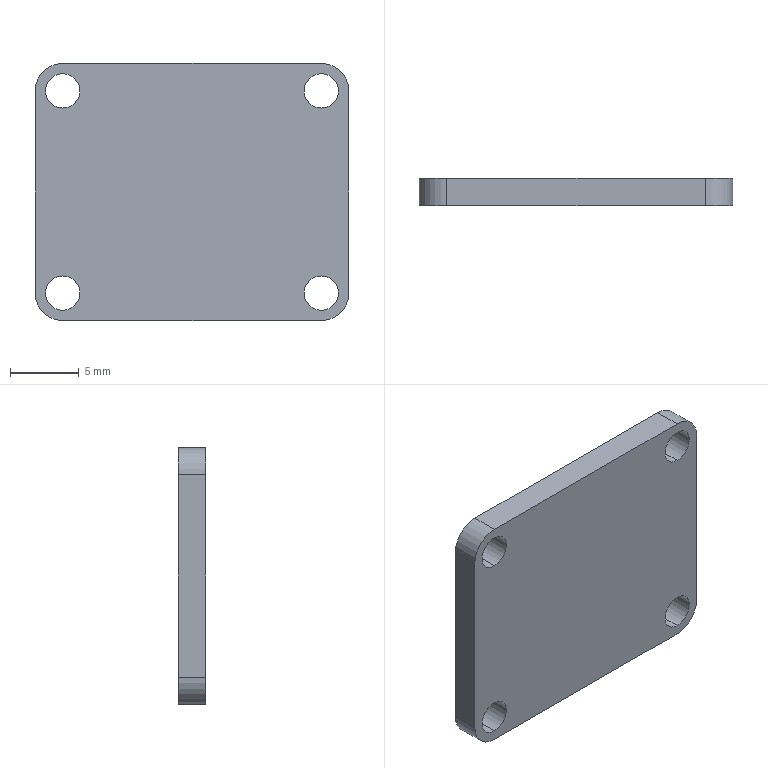Part | SolidWorks | features ICE 5, ExtruThin 1, Fillet 1 | 1 solid | 18 faces | box 22.8 x 2 x 18.7 mm | volume 806.583 mm3 | cylinder 12 | plane 6 | commonest cylinder face diameters 2.5 x8 4 x4
STEP:
#1=CARTESIAN_POINT('',(36.275,113.634,-14.95));
#2=VERTEX_POINT('',#1);
#3=CARTESIAN_POINT('',(36.275,113.634,-12.45));
#4=VERTEX_POINT('',#3);
#5=CARTESIAN_POINT('',(36.275,113.634,-13.7));
#6=DIRECTION('',(0.,1.,0.));
#7=DIRECTION('',(0.,0.,1.));
#8=AXIS2_PLACEMENT_3D('',#5,#6,#7);
#9=CIRCLE('',#8,1.25);
#10=EDGE_CURVE('',#2,#4,#9,.T.);
#11=ORIENTED_EDGE('',*,*,#10,.F.);
#12=CARTESIAN_POINT('',(36.275,115.634,-14.95));
#13=VERTEX_POINT('',#12);
#14=CARTESIAN_POINT('',(36.275,113.634,-14.95));
#15=DIRECTION('',(0.,1.,0.));
#16=VECTOR('',#15,1000.);
#17=LINE('',#14,#16);
#18=EDGE_CURVE('',#2,#13,#17,.T.);
#19=ORIENTED_EDGE('',*,*,#18,.T.);
#20=CARTESIAN_POINT('',(36.275,115.634,-12.45));
#21=VERTEX_POINT('',#20);
#22=CARTESIAN_POINT('',(36.275,115.634,-13.7));
#23=DIRECTION('',(0.,1.,0.));
#24=DIRECTION('',(0.,0.,1.));
#25=AXIS2_PLACEMENT_3D('',#22,#23,#24);
#26=CIRCLE('',#25,1.25);
#27=EDGE_CURVE('',#13,#21,#26,.T.);
#28=ORIENTED_EDGE('',*,*,#27,.T.);
#29=CARTESIAN_POINT('',(36.275,113.634,-12.45));
#30=DIRECTION('',(0.,1.,0.));
#31=VECTOR('',#30,1000.);
#32=LINE('',#29,#31);
#33=EDGE_CURVE('',#4,#21,#32,.T.);
#34=ORIENTED_EDGE('',*,*,#33,.F.);
#35=EDGE_LOOP('',(#11,#19,#28,#34));
#36=FACE_OUTER_BOUND('',#35,.T.);
#37=CARTESIAN_POINT('',(36.275,113.634,-13.7));
#38=DIRECTION('',(0.,1.,0.));
#39=DIRECTION('',(0.,0.,1.));
#40=AXIS2_PLACEMENT_3D('',#37,#38,#39);
#41=CYLINDRICAL_SURFACE('',#40,1.25);
#42=ADVANCED_FACE('',(#36),#41,.F.);
#43=CARTESIAN_POINT('',(36.275,113.634,-0.25));
#44=VERTEX_POINT('',#43);
#45=CARTESIAN_POINT('',(36.275,113.634,2.25));
#46=VERTEX_POINT('',#45);
#47=CARTESIAN_POINT('',(36.275,113.634,1.));
#48=DIRECTION('',(0.,1.,0.));
#49=DIRECTION('',(0.,0.,1.));
#50=AXIS2_PLACEMENT_3D('',#47,#48,#49);
#51=CIRCLE('',#50,1.25);
#52=EDGE_CURVE('',#44,#46,#51,.T.);
#53=ORIENTED_EDGE('',*,*,#52,.F.);
#54=CARTESIAN_POINT('',(36.275,115.634,-0.25));
#55=VERTEX_POINT('',#54);
#56=CARTESIAN_POINT('',(36.275,113.634,-0.25));
#57=DIRECTION('',(0.,1.,0.));
#58=VECTOR('',#57,1000.);
#59=LINE('',#56,#58);
#60=EDGE_CURVE('',#44,#55,#59,.T.);
#61=ORIENTED_EDGE('',*,*,#60,.T.);
#62=CARTESIAN_POINT('',(36.275,115.634,2.25));
#63=VERTEX_POINT('',#62);
#64=CARTESIAN_POINT('',(36.275,115.634,1.));
#65=DIRECTION('',(0.,1.,0.));
#66=DIRECTION('',(0.,0.,1.));
#67=AXIS2_PLACEMENT_3D('',#64,#65,#66);
#68=CIRCLE('',#67,1.25);
#69=EDGE_CURVE('',#55,#63,#68,.T.);
#70=ORIENTED_EDGE('',*,*,#69,.T.);
#71=CARTESIAN_POINT('',(36.275,113.634,2.25));
#72=DIRECTION('',(0.,1.,0.));
#73=VECTOR('',#72,1000.);
#74=LINE('',#71,#73);
#75=EDGE_CURVE('',#46,#63,#74,.T.);
#76=ORIENTED_EDGE('',*,*,#75,.F.);
#77=EDGE_LOOP('',(#53,#61,#70,#76));
#78=FACE_OUTER_BOUND('',#77,.T.);
#79=CARTESIAN_POINT('',(36.275,113.634,1.));
#80=DIRECTION('',(0.,1.,0.));
#81=DIRECTION('',(0.,0.,1.));
#82=AXIS2_PLACEMENT_3D('',#79,#80,#81);
#83=CYLINDRICAL_SURFACE('',#82,1.25);
#84=ADVANCED_FACE('',(#78),#83,.F.);
#85=CARTESIAN_POINT('',(55.075,113.634,-0.25));
#86=VERTEX_POINT('',#85);
#87=CARTESIAN_POINT('',(55.075,113.634,2.25));
#88=VERTEX_POINT('',#87);
#89=CARTESIAN_POINT('',(55.075,113.634,1.));
#90=DIRECTION('',(0.,1.,0.));
#91=DIRECTION('',(0.,0.,1.));
#92=AXIS2_PLACEMENT_3D('',#89,#90,#91);
#93=CIRCLE('',#92,1.25);
#94=EDGE_CURVE('',#86,#88,#93,.T.);
#95=ORIENTED_EDGE('',*,*,#94,.F.);
#96=CARTESIAN_POINT('',(55.075,115.634,-0.25));
#97=VERTEX_POINT('',#96);
#98=CARTESIAN_POINT('',(55.075,113.634,-0.25));
#99=DIRECTION('',(0.,1.,0.));
#100=VECTOR('',#99,1000.);
#101=LINE('',#98,#100);
#102=EDGE_CURVE('',#86,#97,#101,.T.);
#103=ORIENTED_EDGE('',*,*,#102,.T.);
#104=CARTESIAN_POINT('',(55.075,115.634,2.25));
#105=VERTEX_POINT('',#104);
#106=CARTESIAN_POINT('',(55.075,115.634,1.));
#107=DIRECTION('',(0.,1.,0.));
#108=DIRECTION('',(0.,0.,1.));
#109=AXIS2_PLACEMENT_3D('',#106,#107,#108);
#110=CIRCLE('',#109,1.25);
#111=EDGE_CURVE('',#97,#105,#110,.T.);
#112=ORIENTED_EDGE('',*,*,#111,.T.);
#113=CARTESIAN_POINT('',(55.075,113.634,2.25));
#114=DIRECTION('',(0.,1.,0.));
#115=VECTOR('',#114,1000.);
#116=LINE('',#113,#115);
#117=EDGE_CURVE('',#88,#105,#116,.T.);
#118=ORIENTED_EDGE('',*,*,#117,.F.);
#119=EDGE_LOOP('',(#95,#103,#112,#118));
#120=FACE_OUTER_BOUND('',#119,.T.);
#121=CARTESIAN_POINT('',(55.075,113.634,1.));
#122=DIRECTION('',(0.,1.,0.));
#123=DIRECTION('',(0.,0.,1.));
#124=AXIS2_PLACEMENT_3D('',#121,#122,#123);
#125=CYLINDRICAL_SURFACE('',#124,1.25);
#126=ADVANCED_FACE('',(#120),#125,.F.);
#127=CARTESIAN_POINT('',(55.075,113.634,-14.95));
#128=VERTEX_POINT('',#127);
#129=CARTESIAN_POINT('',(55.075,113.634,-12.45));
#130=VERTEX_POINT('',#129);
#131=CARTESIAN_POINT('',(55.075,113.634,-13.7));
#132=DIRECTION('',(0.,1.,0.));
#133=DIRECTION('',(0.,0.,1.));
#134=AXIS2_PLACEMENT_3D('',#131,#132,#133);
#135=CIRCLE('',#134,1.25);
#136=EDGE_CURVE('',#128,#130,#135,.T.);
#137=ORIENTED_EDGE('',*,*,#136,.F.);
#138=CARTESIAN_POINT('',(55.075,115.634,-14.95));
#139=VERTEX_POINT('',#138);
#140=CARTESIAN_POINT('',(55.075,113.634,-14.95));
#141=DIRECTION('',(0.,1.,0.));
#142=VECTOR('',#141,1000.);
#143=LINE('',#140,#142);
#144=EDGE_CURVE('',#128,#139,#143,.T.);
#145=ORIENTED_EDGE('',*,*,#144,.T.);
#146=CARTESIAN_POINT('',(55.075,115.634,-12.45));
#147=VERTEX_POINT('',#146);
#148=CARTESIAN_POINT('',(55.075,115.634,-13.7));
#149=DIRECTION('',(0.,1.,0.));
#150=DIRECTION('',(0.,0.,1.));
#151=AXIS2_PLACEMENT_3D('',#148,#149,#150);
#152=CIRCLE('',#151,1.25);
#153=EDGE_CURVE('',#139,#147,#152,.T.);
#154=ORIENTED_EDGE('',*,*,#153,.T.);
#155=CARTESIAN_POINT('',(55.075,113.634,-12.45));
#156=DIRECTION('',(0.,1.,0.));
#157=VECTOR('',#156,1000.);
#158=LINE('',#155,#157);
#159=EDGE_CURVE('',#130,#147,#158,.T.);
#160=ORIENTED_EDGE('',*,*,#159,.F.);
#161=EDGE_LOOP('',(#137,#145,#154,#160));
#162=FACE_OUTER_BOUND('',#161,.T.);
#163=CARTESIAN_POINT('',(55.075,113.634,-13.7));
#164=DIRECTION('',(0.,1.,0.));
#165=DIRECTION('',(0.,0.,1.));
#166=AXIS2_PLACEMENT_3D('',#163,#164,#165);
#167=CYLINDRICAL_SURFACE('',#166,1.25);
#168=ADVANCED_FACE('',(#162),#167,.F.);
#169=CARTESIAN_POINT('',(57.075,115.634,1.));
#170=VERTEX_POINT('',#169);
#171=CARTESIAN_POINT('',(57.075,115.634,-13.7));
#172=VERTEX_POINT('',#171);
#173=CARTESIAN_POINT('',(57.075,115.634,-15.7));
#174=DIRECTION('',(0.,0.,-1.));
#175=VECTOR('',#174,1000.);
#176=LINE('',#173,#175);
#177=EDGE_CURVE('',#170,#172,#176,.T.);
#178=ORIENTED_EDGE('',*,*,#177,.F.);
#179=CARTESIAN_POINT('',(57.075,113.634,1.));
#180=VERTEX_POINT('',#179);
#181=CARTESIAN_POINT('',(57.075,115.634,1.));
#182=DIRECTION('',(0.,-1.,0.));
#183=VECTOR('',#182,1000.);
#184=LINE('',#181,#183);
#185=EDGE_CURVE('',#170,#180,#184,.T.);
#186=ORIENTED_EDGE('',*,*,#185,.T.);
#187=CARTESIAN_POINT('',(57.075,113.634,-13.7));
#188=VERTEX_POINT('',#187);
#189=CARTESIAN_POINT('',(57.075,113.634,-15.7));
#190=DIRECTION('',(0.,0.,-1.));
#191=VECTOR('',#190,1000.);
#192=LINE('',#189,#191);
#193=EDGE_CURVE('',#180,#188,#192,.T.);
#194=ORIENTED_EDGE('',*,*,#193,.T.);
#195=CARTESIAN_POINT('',(57.075,115.634,-13.7));
#196=DIRECTION('',(0.,1.,0.));
#197=VECTOR('',#196,1000.);
#198=LINE('',#195,#197);
#199=EDGE_CURVE('',#188,#172,#198,.T.);
#200=ORIENTED_EDGE('',*,*,#199,.T.);
#201=EDGE_LOOP('',(#178,#186,#194,#200));
#202=FACE_OUTER_BOUND('',#201,.T.);
#203=CARTESIAN_POINT('',(57.075,115.634,-15.7));
#204=DIRECTION('',(-1.,0.,0.));
#205=DIRECTION('',(0.,0.,1.));
#206=AXIS2_PLACEMENT_3D('',#203,#204,#205);
#207=PLANE('',#206);
#208=ADVANCED_FACE('',(#202),#207,.F.);
#209=CARTESIAN_POINT('',(55.075,113.634,-15.7));
#210=VERTEX_POINT('',#209);
#211=CARTESIAN_POINT('',(36.275,113.634,-15.7));
#212=VERTEX_POINT('',#211);
#213=CARTESIAN_POINT('',(57.075,113.634,-15.7));
#214=DIRECTION('',(-1.,0.,0.));
#215=VECTOR('',#214,1000.);
#216=LINE('',#213,#215);
#217=EDGE_CURVE('',#210,#212,#216,.T.);
#218=ORIENTED_EDGE('',*,*,#217,.T.);
#219=CARTESIAN_POINT('',(36.275,115.634,-15.7));
#220=VERTEX_POINT('',#219);
#221=CARTESIAN_POINT('',(36.275,115.634,-15.7));
#222=DIRECTION('',(0.,1.,0.));
#223=VECTOR('',#222,1000.);
#224=LINE('',#221,#223);
#225=EDGE_CURVE('',#212,#220,#224,.T.);
#226=ORIENTED_EDGE('',*,*,#225,.T.);
#227=CARTESIAN_POINT('',(55.075,115.634,-15.7));
#228=VERTEX_POINT('',#227);
#229=CARTESIAN_POINT('',(57.075,115.634,-15.7));
#230=DIRECTION('',(-1.,0.,0.));
#231=VECTOR('',#230,1000.);
#232=LINE('',#229,#231);
#233=EDGE_CURVE('',#228,#220,#232,.T.);
#234=ORIENTED_EDGE('',*,*,#233,.F.);
#235=CARTESIAN_POINT('',(55.075,115.634,-15.7));
#236=DIRECTION('',(0.,-1.,0.));
#237=VECTOR('',#236,1000.);
#238=LINE('',#235,#237);
#239=EDGE_CURVE('',#228,#210,#238,.T.);
#240=ORIENTED_EDGE('',*,*,#239,.T.);
#241=EDGE_LOOP('',(#218,#226,#234,#240));
#242=FACE_OUTER_BOUND('',#241,.T.);
#243=CARTESIAN_POINT('',(57.075,115.634,-15.7));
#244=DIRECTION('',(0.,0.,1.));
#245=DIRECTION('',(1.,0.,0.));
#246=AXIS2_PLACEMENT_3D('',#243,#244,#245);
#247=PLANE('',#246);
#248=ADVANCED_FACE('',(#242),#247,.F.);
#249=CARTESIAN_POINT('',(34.275,113.634,-13.7));
#250=VERTEX_POINT('',#249);
#251=CARTESIAN_POINT('',(34.275,113.634,1.));
#252=VERTEX_POINT('',#251);
#253=CARTESIAN_POINT('',(34.275,113.634,-15.7));
#254=DIRECTION('',(0.,0.,1.));
#255=VECTOR('',#254,1000.);
#256=LINE('',#253,#255);
#257=EDGE_CURVE('',#250,#252,#256,.T.);
#258=ORIENTED_EDGE('',*,*,#257,.T.);
#259=CARTESIAN_POINT('',(34.275,115.634,1.));
#260=VERTEX_POINT('',#259);
#261=CARTESIAN_POINT('',(34.275,115.634,1.));
#262=DIRECTION('',(0.,1.,0.));
#263=VECTOR('',#262,1000.);
#264=LINE('',#261,#263);
#265=EDGE_CURVE('',#252,#260,#264,.T.);
#266=ORIENTED_EDGE('',*,*,#265,.T.);
#267=CARTESIAN_POINT('',(34.275,115.634,-13.7));
#268=VERTEX_POINT('',#267);
#269=CARTESIAN_POINT('',(34.275,115.634,-15.7));
#270=DIRECTION('',(0.,0.,1.));
#271=VECTOR('',#270,1000.);
#272=LINE('',#269,#271);
#273=EDGE_CURVE('',#268,#260,#272,.T.);
#274=ORIENTED_EDGE('',*,*,#273,.F.);
#275=CARTESIAN_POINT('',(34.275,115.634,-13.7));
#276=DIRECTION('',(0.,-1.,0.));
#277=VECTOR('',#276,1000.);
#278=LINE('',#275,#277);
#279=EDGE_CURVE('',#268,#250,#278,.T.);
#280=ORIENTED_EDGE('',*,*,#279,.T.);
#281=EDGE_LOOP('',(#258,#266,#274,#280));
#282=FACE_OUTER_BOUND('',#281,.T.);
#283=CARTESIAN_POINT('',(34.275,115.634,-15.7));
#284=DIRECTION('',(1.,0.,0.));
#285=DIRECTION('',(0.,0.,-1.));
#286=AXIS2_PLACEMENT_3D('',#283,#284,#285);
#287=PLANE('',#286);
#288=ADVANCED_FACE('',(#282),#287,.F.);
#289=CARTESIAN_POINT('',(36.275,113.634,3.));
#290=VERTEX_POINT('',#289);
#291=CARTESIAN_POINT('',(55.075,113.634,3.));
#292=VERTEX_POINT('',#291);
#293=CARTESIAN_POINT('',(57.075,113.634,3.));
#294=DIRECTION('',(1.,0.,0.));
#295=VECTOR('',#294,1000.);
#296=LINE('',#293,#295);
#297=EDGE_CURVE('',#290,#292,#296,.T.);
#298=ORIENTED_EDGE('',*,*,#297,.T.);
#299=CARTESIAN_POINT('',(55.075,115.634,3.));
#300=VERTEX_POINT('',#299);
#301=CARTESIAN_POINT('',(55.075,115.634,3.));
#302=DIRECTION('',(0.,1.,0.));
#303=VECTOR('',#302,1000.);
#304=LINE('',#301,#303);
#305=EDGE_CURVE('',#292,#300,#304,.T.);
#306=ORIENTED_EDGE('',*,*,#305,.T.);
#307=CARTESIAN_POINT('',(36.275,115.634,3.));
#308=VERTEX_POINT('',#307);
#309=CARTESIAN_POINT('',(57.075,115.634,3.));
#310=DIRECTION('',(1.,0.,0.));
#311=VECTOR('',#310,1000.);
#312=LINE('',#309,#311);
#313=EDGE_CURVE('',#308,#300,#312,.T.);
#314=ORIENTED_EDGE('',*,*,#313,.F.);
#315=CARTESIAN_POINT('',(36.275,115.634,3.));
#316=DIRECTION('',(0.,-1.,0.));
#317=VECTOR('',#316,1000.);
#318=LINE('',#315,#317);
#319=EDGE_CURVE('',#308,#290,#318,.T.);
#320=ORIENTED_EDGE('',*,*,#319,.T.);
#321=EDGE_LOOP('',(#298,#306,#314,#320));
#322=FACE_OUTER_BOUND('',#321,.T.);
#323=CARTESIAN_POINT('',(57.075,115.634,3.));
#324=DIRECTION('',(0.,0.,-1.));
#325=DIRECTION('',(-1.,0.,0.));
#326=AXIS2_PLACEMENT_3D('',#323,#324,#325);
#327=PLANE('',#326);
#328=ADVANCED_FACE('',(#322),#327,.F.);
#329=CARTESIAN_POINT('',(36.275,115.634,-13.7));
#330=DIRECTION('',(0.,1.,0.));
#331=DIRECTION('',(0.,0.,1.));
#332=AXIS2_PLACEMENT_3D('',#329,#330,#331);
#333=CIRCLE('',#332,1.25);
#334=EDGE_CURVE('',#21,#13,#333,.T.);
#335=ORIENTED_EDGE('',*,*,#334,.F.);
#336=ORIENTED_EDGE('',*,*,#27,.F.);
#337=EDGE_LOOP('',(#335,#336));
#338=FACE_BOUND('',#337,.T.);
#339=CARTESIAN_POINT('',(36.275,115.634,1.));
#340=DIRECTION('',(0.,1.,0.));
#341=DIRECTION('',(0.,0.,1.));
#342=AXIS2_PLACEMENT_3D('',#339,#340,#341);
#343=CIRCLE('',#342,1.25);
#344=EDGE_CURVE('',#63,#55,#343,.T.);
#345=ORIENTED_EDGE('',*,*,#344,.F.);
#346=ORIENTED_EDGE('',*,*,#69,.F.);
#347=EDGE_LOOP('',(#345,#346));
#348=FACE_BOUND('',#347,.T.);
#349=CARTESIAN_POINT('',(55.075,115.634,1.));
#350=DIRECTION('',(0.,1.,0.));
#351=DIRECTION('',(0.,0.,1.));
#352=AXIS2_PLACEMENT_3D('',#349,#350,#351);
#353=CIRCLE('',#352,1.25);
#354=EDGE_CURVE('',#105,#97,#353,.T.);
#355=ORIENTED_EDGE('',*,*,#354,.F.);
#356=ORIENTED_EDGE('',*,*,#111,.F.);
#357=EDGE_LOOP('',(#355,#356));
#358=FACE_BOUND('',#357,.T.);
#359=CARTESIAN_POINT('',(55.075,115.634,-13.7));
#360=DIRECTION('',(0.,1.,0.));
#361=DIRECTION('',(0.,0.,1.));
#362=AXIS2_PLACEMENT_3D('',#359,#360,#361);
#363=CIRCLE('',#362,1.25);
#364=EDGE_CURVE('',#147,#139,#363,.T.);
#365=ORIENTED_EDGE('',*,*,#364,.F.);
#366=ORIENTED_EDGE('',*,*,#153,.F.);
#367=EDGE_LOOP('',(#365,#366));
#368=FACE_BOUND('',#367,.T.);
#369=ORIENTED_EDGE('',*,*,#313,.T.);
#370=CARTESIAN_POINT('',(55.075,115.634,1.));
#371=DIRECTION('',(0.,1.,0.));
#372=DIRECTION('',(0.,0.,-1.));
#373=AXIS2_PLACEMENT_3D('',#370,#371,#372);
#374=CIRCLE('',#373,2.);
#375=EDGE_CURVE('',#300,#170,#374,.T.);
#376=ORIENTED_EDGE('',*,*,#375,.T.);
#377=ORIENTED_EDGE('',*,*,#177,.T.);
#378=CARTESIAN_POINT('',(55.075,115.634,-13.7));
#379=DIRECTION('',(0.,1.,0.));
#380=DIRECTION('',(0.,0.,-1.));
#381=AXIS2_PLACEMENT_3D('',#378,#379,#380);
#382=CIRCLE('',#381,2.);
#383=EDGE_CURVE('',#172,#228,#382,.T.);
#384=ORIENTED_EDGE('',*,*,#383,.T.);
#385=ORIENTED_EDGE('',*,*,#233,.T.);
#386=CARTESIAN_POINT('',(36.275,115.634,-13.7));
#387=DIRECTION('',(0.,1.,0.));
#388=DIRECTION('',(0.,0.,-1.));
#389=AXIS2_PLACEMENT_3D('',#386,#387,#388);
#390=CIRCLE('',#389,2.);
#391=EDGE_CURVE('',#220,#268,#390,.T.);
#392=ORIENTED_EDGE('',*,*,#391,.T.);
#393=ORIENTED_EDGE('',*,*,#273,.T.);
#394=CARTESIAN_POINT('',(36.275,115.634,1.));
#395=DIRECTION('',(0.,1.,0.));
#396=DIRECTION('',(0.,0.,-1.));
#397=AXIS2_PLACEMENT_3D('',#394,#395,#396);
#398=CIRCLE('',#397,2.);
#399=EDGE_CURVE('',#260,#308,#398,.T.);
#400=ORIENTED_EDGE('',*,*,#399,.T.);
#401=EDGE_LOOP('',(#369,#376,#377,#384,#385,#392,#393,#400));
#402=FACE_OUTER_BOUND('',#401,.T.);
#403=CARTESIAN_POINT('',(0.,115.634,0.));
#404=DIRECTION('',(0.,-1.,0.));
#405=DIRECTION('',(0.,0.,-1.));
#406=AXIS2_PLACEMENT_3D('',#403,#404,#405);
#407=PLANE('',#406);
#408=ADVANCED_FACE('',(#338,#348,#358,#368,#402),#407,.F.);
#409=CARTESIAN_POINT('',(55.075,113.634,-13.7));
#410=DIRECTION('',(0.,1.,0.));
#411=DIRECTION('',(0.,0.,1.));
#412=AXIS2_PLACEMENT_3D('',#409,#410,#411);
#413=CIRCLE('',#412,1.25);
#414=EDGE_CURVE('',#130,#128,#413,.T.);
#415=ORIENTED_EDGE('',*,*,#414,.T.);
#416=ORIENTED_EDGE('',*,*,#136,.T.);
#417=EDGE_LOOP('',(#415,#416));
#418=FACE_BOUND('',#417,.T.);
#419=CARTESIAN_POINT('',(55.075,113.634,1.));
#420=DIRECTION('',(0.,1.,0.));
#421=DIRECTION('',(0.,0.,1.));
#422=AXIS2_PLACEMENT_3D('',#419,#420,#421);
#423=CIRCLE('',#422,1.25);
#424=EDGE_CURVE('',#88,#86,#423,.T.);
#425=ORIENTED_EDGE('',*,*,#424,.T.);
#426=ORIENTED_EDGE('',*,*,#94,.T.);
#427=EDGE_LOOP('',(#425,#426));
#428=FACE_BOUND('',#427,.T.);
#429=ORIENTED_EDGE('',*,*,#217,.F.);
#430=CARTESIAN_POINT('',(55.075,113.634,-13.7));
#431=DIRECTION('',(0.,-1.,0.));
#432=DIRECTION('',(0.,0.,-1.));
#433=AXIS2_PLACEMENT_3D('',#430,#431,#432);
#434=CIRCLE('',#433,2.);
#435=EDGE_CURVE('',#210,#188,#434,.T.);
#436=ORIENTED_EDGE('',*,*,#435,.T.);
#437=ORIENTED_EDGE('',*,*,#193,.F.);
#438=CARTESIAN_POINT('',(55.075,113.634,1.));
#439=DIRECTION('',(0.,-1.,0.));
#440=DIRECTION('',(0.,0.,-1.));
#441=AXIS2_PLACEMENT_3D('',#438,#439,#440);
#442=CIRCLE('',#441,2.);
#443=EDGE_CURVE('',#180,#292,#442,.T.);
#444=ORIENTED_EDGE('',*,*,#443,.T.);
#445=ORIENTED_EDGE('',*,*,#297,.F.);
#446=CARTESIAN_POINT('',(36.275,113.634,1.));
#447=DIRECTION('',(0.,-1.,0.));
#448=DIRECTION('',(0.,0.,-1.));
#449=AXIS2_PLACEMENT_3D('',#446,#447,#448);
#450=CIRCLE('',#449,2.);
#451=EDGE_CURVE('',#290,#252,#450,.T.);
#452=ORIENTED_EDGE('',*,*,#451,.T.);
#453=ORIENTED_EDGE('',*,*,#257,.F.);
#454=CARTESIAN_POINT('',(36.275,113.634,-13.7));
#455=DIRECTION('',(0.,-1.,0.));
#456=DIRECTION('',(0.,0.,-1.));
#457=AXIS2_PLACEMENT_3D('',#454,#455,#456);
#458=CIRCLE('',#457,2.);
#459=EDGE_CURVE('',#250,#212,#458,.T.);
#460=ORIENTED_EDGE('',*,*,#459,.T.);
#461=EDGE_LOOP('',(#429,#436,#437,#444,#445,#452,#453,#460));
#462=FACE_OUTER_BOUND('',#461,.T.);
#463=CARTESIAN_POINT('',(36.275,113.634,-13.7));
#464=DIRECTION('',(0.,1.,0.));
#465=DIRECTION('',(0.,0.,1.));
#466=AXIS2_PLACEMENT_3D('',#463,#464,#465);
#467=CIRCLE('',#466,1.25);
#468=EDGE_CURVE('',#4,#2,#467,.T.);
#469=ORIENTED_EDGE('',*,*,#468,.T.);
#470=ORIENTED_EDGE('',*,*,#10,.T.);
#471=EDGE_LOOP('',(#469,#470));
#472=FACE_BOUND('',#471,.T.);
#473=CARTESIAN_POINT('',(36.275,113.634,1.));
#474=DIRECTION('',(0.,1.,0.));
#475=DIRECTION('',(0.,0.,1.));
#476=AXIS2_PLACEMENT_3D('',#473,#474,#475);
#477=CIRCLE('',#476,1.25);
#478=EDGE_CURVE('',#46,#44,#477,.T.);
#479=ORIENTED_EDGE('',*,*,#478,.T.);
#480=ORIENTED_EDGE('',*,*,#52,.T.);
#481=EDGE_LOOP('',(#479,#480));
#482=FACE_BOUND('',#481,.T.);
#483=CARTESIAN_POINT('',(0.,113.634,0.));
#484=DIRECTION('',(0.,-1.,0.));
#485=DIRECTION('',(0.,0.,-1.));
#486=AXIS2_PLACEMENT_3D('',#483,#484,#485);
#487=PLANE('',#486);
#488=ADVANCED_FACE('',(#418,#428,#462,#472,#482),#487,.T.);
#489=ORIENTED_EDGE('',*,*,#375,.F.);
#490=ORIENTED_EDGE('',*,*,#305,.F.);
#491=ORIENTED_EDGE('',*,*,#443,.F.);
#492=ORIENTED_EDGE('',*,*,#185,.F.);
#493=EDGE_LOOP('',(#489,#490,#491,#492));
#494=FACE_OUTER_BOUND('',#493,.T.);
#495=CARTESIAN_POINT('',(55.075,115.634,1.));
#496=DIRECTION('',(0.,-1.,0.));
#497=DIRECTION('',(0.,0.,-1.));
#498=AXIS2_PLACEMENT_3D('',#495,#496,#497);
#499=CYLINDRICAL_SURFACE('',#498,2.);
#500=ADVANCED_FACE('',(#494),#499,.T.);
#501=ORIENTED_EDGE('',*,*,#399,.F.);
#502=ORIENTED_EDGE('',*,*,#265,.F.);
#503=ORIENTED_EDGE('',*,*,#451,.F.);
#504=ORIENTED_EDGE('',*,*,#319,.F.);
#505=EDGE_LOOP('',(#501,#502,#503,#504));
#506=FACE_OUTER_BOUND('',#505,.T.);
#507=CARTESIAN_POINT('',(36.275,115.634,1.));
#508=DIRECTION('',(0.,-1.,0.));
#509=DIRECTION('',(0.,0.,-1.));
#510=AXIS2_PLACEMENT_3D('',#507,#508,#509);
#511=CYLINDRICAL_SURFACE('',#510,2.);
#512=ADVANCED_FACE('',(#506),#511,.T.);
#513=ORIENTED_EDGE('',*,*,#391,.F.);
#514=ORIENTED_EDGE('',*,*,#225,.F.);
#515=ORIENTED_EDGE('',*,*,#459,.F.);
#516=ORIENTED_EDGE('',*,*,#279,.F.);
#517=EDGE_LOOP('',(#513,#514,#515,#516));
#518=FACE_OUTER_BOUND('',#517,.T.);
#519=CARTESIAN_POINT('',(36.275,115.634,-13.7));
#520=DIRECTION('',(0.,-1.,0.));
#521=DIRECTION('',(0.,0.,-1.));
#522=AXIS2_PLACEMENT_3D('',#519,#520,#521);
#523=CYLINDRICAL_SURFACE('',#522,2.);
#524=ADVANCED_FACE('',(#518),#523,.T.);
#525=ORIENTED_EDGE('',*,*,#383,.F.);
#526=ORIENTED_EDGE('',*,*,#199,.F.);
#527=ORIENTED_EDGE('',*,*,#435,.F.);
#528=ORIENTED_EDGE('',*,*,#239,.F.);
#529=EDGE_LOOP('',(#525,#526,#527,#528));
#530=FACE_OUTER_BOUND('',#529,.T.);
#531=CARTESIAN_POINT('',(55.075,115.634,-13.7));
#532=DIRECTION('',(0.,-1.,0.));
#533=DIRECTION('',(0.,0.,-1.));
#534=AXIS2_PLACEMENT_3D('',#531,#532,#533);
#535=CYLINDRICAL_SURFACE('',#534,2.);
#536=ADVANCED_FACE('',(#530),#535,.T.);
#537=ORIENTED_EDGE('',*,*,#144,.F.);
#538=ORIENTED_EDGE('',*,*,#414,.F.);
#539=ORIENTED_EDGE('',*,*,#159,.T.);
#540=ORIENTED_EDGE('',*,*,#364,.T.);
#541=EDGE_LOOP('',(#537,#538,#539,#540));
#542=FACE_OUTER_BOUND('',#541,.T.);
#543=CARTESIAN_POINT('',(55.075,113.634,-13.7));
#544=DIRECTION('',(0.,1.,0.));
#545=DIRECTION('',(0.,0.,1.));
#546=AXIS2_PLACEMENT_3D('',#543,#544,#545);
#547=CYLINDRICAL_SURFACE('',#546,1.25);
#548=ADVANCED_FACE('',(#542),#547,.F.);
#549=ORIENTED_EDGE('',*,*,#102,.F.);
#550=ORIENTED_EDGE('',*,*,#424,.F.);
#551=ORIENTED_EDGE('',*,*,#117,.T.);
#552=ORIENTED_EDGE('',*,*,#354,.T.);
#553=EDGE_LOOP('',(#549,#550,#551,#552));
#554=FACE_OUTER_BOUND('',#553,.T.);
#555=CARTESIAN_POINT('',(55.075,113.634,1.));
#556=DIRECTION('',(0.,1.,0.));
#557=DIRECTION('',(0.,0.,1.));
#558=AXIS2_PLACEMENT_3D('',#555,#556,#557);
#559=CYLINDRICAL_SURFACE('',#558,1.25);
#560=ADVANCED_FACE('',(#554),#559,.F.);
#561=ORIENTED_EDGE('',*,*,#60,.F.);
#562=ORIENTED_EDGE('',*,*,#478,.F.);
#563=ORIENTED_EDGE('',*,*,#75,.T.);
#564=ORIENTED_EDGE('',*,*,#344,.T.);
#565=EDGE_LOOP('',(#561,#562,#563,#564));
#566=FACE_OUTER_BOUND('',#565,.T.);
#567=CARTESIAN_POINT('',(36.275,113.634,1.));
#568=DIRECTION('',(0.,1.,0.));
#569=DIRECTION('',(0.,0.,1.));
#570=AXIS2_PLACEMENT_3D('',#567,#568,#569);
#571=CYLINDRICAL_SURFACE('',#570,1.25);
#572=ADVANCED_FACE('',(#566),#571,.F.);
#573=ORIENTED_EDGE('',*,*,#18,.F.);
#574=ORIENTED_EDGE('',*,*,#468,.F.);
#575=ORIENTED_EDGE('',*,*,#33,.T.);
#576=ORIENTED_EDGE('',*,*,#334,.T.);
#577=EDGE_LOOP('',(#573,#574,#575,#576));
#578=FACE_OUTER_BOUND('',#577,.T.);
#579=CARTESIAN_POINT('',(36.275,113.634,-13.7));
#580=DIRECTION('',(0.,1.,0.));
#581=DIRECTION('',(0.,0.,1.));
#582=AXIS2_PLACEMENT_3D('',#579,#580,#581);
#583=CYLINDRICAL_SURFACE('',#582,1.25);
#584=ADVANCED_FACE('',(#578),#583,.F.);
#585=CLOSED_SHELL('',(#42,#84,#126,#168,#208,#248,#288,#328,#408,#488,#500,#512,#524,#536,#548,#560,#572,#584));
#586=MANIFOLD_SOLID_BREP('',#585);
#587=CARTESIAN_POINT('',(0.,0.,0.));
#588=DIRECTION('',(0.,0.,1.));
#589=DIRECTION('',(1.,0.,0.));
#590=AXIS2_PLACEMENT_3D('',#587,#588,#589);
#591=(LENGTH_UNIT()NAMED_UNIT(*)SI_UNIT(.MILLI.,.METRE.));
#592=UNCERTAINTY_MEASURE_WITH_UNIT(LENGTH_MEASURE(0.00001),#591,'','');
#593=(NAMED_UNIT(*)PLANE_ANGLE_UNIT()SI_UNIT($,.RADIAN.));
#594=(NAMED_UNIT(*)SI_UNIT($,.STERADIAN.)SOLID_ANGLE_UNIT());
#595=(GEOMETRIC_REPRESENTATION_CONTEXT(3)GLOBAL_UNCERTAINTY_ASSIGNED_CONTEXT((#592))GLOBAL_UNIT_ASSIGNED_CONTEXT((#591,#593,#594))REPRESENTATION_CONTEXT('',''));
#596=ADVANCED_BREP_SHAPE_REPRESENTATION('',(#586,#590),#595);